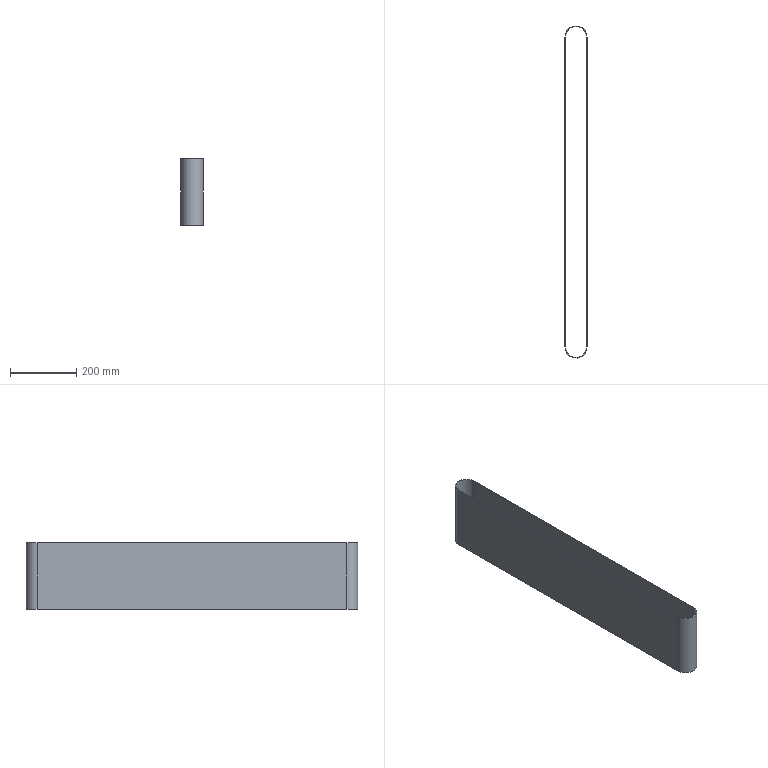Part | STEP file | MM-P41130-13_1 | 1 solid | 10 faces | box 67 x 999.5 x 200 mm | volume 621232 mm3 | plane 6 | cylinder 4 | commonest cylinder face diameters 64 x2 67 x2
STEP:
#1=CARTESIAN_POINT('',(0.,0.,0.));
#2=DIRECTION('',(0.,0.,1.));
#3=DIRECTION('',(1.,0.,0.));
#4=AXIS2_PLACEMENT_3D('',#1,#2,#3);
#5=CARTESIAN_POINT('',(-17.,-947.5,100.));
#6=VERTEX_POINT('',#5);
#7=CARTESIAN_POINT('',(-17.,-947.5,-100.));
#8=VERTEX_POINT('',#7);
#9=CARTESIAN_POINT('',(-17.,-947.5,100.));
#10=DIRECTION('',(0.,0.,-1.));
#11=VECTOR('',#10,1.);
#12=LINE('',#9,#11);
#13=CARTESIAN_POINT('',(-17.,-15.,100.));
#14=DIRECTION('',(1.,-0.000000039,0.));
#15=DIRECTION('',(0.000000039,1.,0.));
#16=AXIS2_PLACEMENT_3D('',#13,#14,#15);
#17=PLANE('',#16);
#18=CARTESIAN_POINT('',(-932.5,0.));
#19=DIRECTION('',(0.,-1.));
#20=VECTOR('',#19,1.);
#21=LINE('',#18,#20);
#22=(GEOMETRIC_REPRESENTATION_CONTEXT(2)PARAMETRIC_REPRESENTATION_CONTEXT()REPRESENTATION_CONTEXT('',''));
#23=DEFINITIONAL_REPRESENTATION('',(#21),#22);
#24=PCURVE('',#17,#23);
#25=CARTESIAN_POINT('',(16.5,-947.5,100.));
#26=DIRECTION('',(0.,0.,1.));
#27=DIRECTION('',(1.,0.,0.));
#28=AXIS2_PLACEMENT_3D('',#25,#26,#27);
#29=CYLINDRICAL_SURFACE('',#28,33.5);
#30=CARTESIAN_POINT('',(3.142,0.));
#31=DIRECTION('',(0.,-1.));
#32=VECTOR('',#31,1.);
#33=LINE('',#30,#32);
#34=(GEOMETRIC_REPRESENTATION_CONTEXT(2)PARAMETRIC_REPRESENTATION_CONTEXT()REPRESENTATION_CONTEXT('',''));
#35=DEFINITIONAL_REPRESENTATION('',(#33),#34);
#36=PCURVE('',#29,#35);
#37=SURFACE_CURVE('',#12,(#24,#36),.PCURVE_S1.);
#38=EDGE_CURVE('',#6,#8,#37,.T.);
#39=ORIENTED_EDGE('',*,*,#38,.F.);
#40=CARTESIAN_POINT('',(-17.,-15.,100.));
#41=VERTEX_POINT('',#40);
#42=CARTESIAN_POINT('',(-17.,-15.,100.));
#43=DIRECTION('',(-0.000000039,-1.,0.));
#44=VECTOR('',#43,1.);
#45=LINE('',#42,#44);
#46=CARTESIAN_POINT('',(0.,0.));
#47=DIRECTION('',(-1.,0.));
#48=VECTOR('',#47,1.);
#49=LINE('',#46,#48);
#50=(GEOMETRIC_REPRESENTATION_CONTEXT(2)PARAMETRIC_REPRESENTATION_CONTEXT()REPRESENTATION_CONTEXT('',''));
#51=DEFINITIONAL_REPRESENTATION('',(#49),#50);
#52=PCURVE('',#17,#51);
#53=CARTESIAN_POINT('',(16.5,-15.,100.));
#54=DIRECTION('',(0.,0.,-1.));
#55=DIRECTION('',(-1.,0.,0.));
#56=AXIS2_PLACEMENT_3D('',#53,#54,#55);
#57=PLANE('',#56);
#58=CARTESIAN_POINT('',(33.5,0.00000132));
#59=DIRECTION('',(0.000000039,-1.));
#60=VECTOR('',#59,1.);
#61=LINE('',#58,#60);
#62=(GEOMETRIC_REPRESENTATION_CONTEXT(2)PARAMETRIC_REPRESENTATION_CONTEXT()REPRESENTATION_CONTEXT('',''));
#63=DEFINITIONAL_REPRESENTATION('',(#61),#62);
#64=PCURVE('',#57,#63);
#65=SURFACE_CURVE('',#45,(#52,#64),.PCURVE_S1.);
#66=EDGE_CURVE('',#41,#6,#65,.T.);
#67=ORIENTED_EDGE('',*,*,#66,.F.);
#68=CARTESIAN_POINT('',(-17.,-15.,-100.));
#69=VERTEX_POINT('',#68);
#70=CARTESIAN_POINT('',(-17.,-15.,100.));
#71=DIRECTION('',(0.,0.,1.));
#72=VECTOR('',#71,1.);
#73=LINE('',#70,#72);
#74=CARTESIAN_POINT('',(0.,0.));
#75=DIRECTION('',(0.,1.));
#76=VECTOR('',#75,1.);
#77=LINE('',#74,#76);
#78=(GEOMETRIC_REPRESENTATION_CONTEXT(2)PARAMETRIC_REPRESENTATION_CONTEXT()REPRESENTATION_CONTEXT('',''));
#79=DEFINITIONAL_REPRESENTATION('',(#77),#78);
#80=PCURVE('',#17,#79);
#81=CARTESIAN_POINT('',(16.5,-15.,100.));
#82=DIRECTION('',(0.,0.,1.));
#83=DIRECTION('',(1.,0.,0.));
#84=AXIS2_PLACEMENT_3D('',#81,#82,#83);
#85=CYLINDRICAL_SURFACE('',#84,33.5);
#86=CARTESIAN_POINT('',(3.142,0.));
#87=DIRECTION('',(0.,1.));
#88=VECTOR('',#87,1.);
#89=LINE('',#86,#88);
#90=(GEOMETRIC_REPRESENTATION_CONTEXT(2)PARAMETRIC_REPRESENTATION_CONTEXT()REPRESENTATION_CONTEXT('',''));
#91=DEFINITIONAL_REPRESENTATION('',(#89),#90);
#92=PCURVE('',#85,#91);
#93=SURFACE_CURVE('',#73,(#80,#92),.PCURVE_S1.);
#94=EDGE_CURVE('',#69,#41,#93,.T.);
#95=ORIENTED_EDGE('',*,*,#94,.F.);
#96=CARTESIAN_POINT('',(-17.,-15.,-100.));
#97=DIRECTION('',(0.000000039,1.,0.));
#98=VECTOR('',#97,1.);
#99=LINE('',#96,#98);
#100=CARTESIAN_POINT('',(0.,-200.));
#101=DIRECTION('',(1.,0.));
#102=VECTOR('',#101,1.);
#103=LINE('',#100,#102);
#104=(GEOMETRIC_REPRESENTATION_CONTEXT(2)PARAMETRIC_REPRESENTATION_CONTEXT()REPRESENTATION_CONTEXT('',''));
#105=DEFINITIONAL_REPRESENTATION('',(#103),#104);
#106=PCURVE('',#17,#105);
#107=CARTESIAN_POINT('',(16.5,-15.,-100.));
#108=DIRECTION('',(0.,0.,-1.));
#109=DIRECTION('',(-1.,0.,0.));
#110=AXIS2_PLACEMENT_3D('',#107,#108,#109);
#111=PLANE('',#110);
#112=CARTESIAN_POINT('',(33.5,0.00000132));
#113=DIRECTION('',(-0.000000039,1.));
#114=VECTOR('',#113,1.);
#115=LINE('',#112,#114);
#116=(GEOMETRIC_REPRESENTATION_CONTEXT(2)PARAMETRIC_REPRESENTATION_CONTEXT()REPRESENTATION_CONTEXT('',''));
#117=DEFINITIONAL_REPRESENTATION('',(#115),#116);
#118=PCURVE('',#111,#117);
#119=SURFACE_CURVE('',#99,(#106,#118),.PCURVE_S1.);
#120=EDGE_CURVE('',#8,#69,#119,.T.);
#121=ORIENTED_EDGE('',*,*,#120,.F.);
#122=EDGE_LOOP('',(#39,#67,#95,#121));
#123=FACE_BOUND('',#122,.T.);
#124=ADVANCED_FACE('',(#123),#17,.F.);
#125=CARTESIAN_POINT('',(-15.5,-15.,-100.));
#126=VERTEX_POINT('',#125);
#127=CARTESIAN_POINT('',(-15.5,-947.5,-100.));
#128=VERTEX_POINT('',#127);
#129=CARTESIAN_POINT('',(-15.5,-15.,-100.));
#130=DIRECTION('',(-0.000000039,-1.,0.));
#131=VECTOR('',#130,1.);
#132=LINE('',#129,#131);
#133=CARTESIAN_POINT('',(32.,0.000001261));
#134=DIRECTION('',(0.000000039,-1.));
#135=VECTOR('',#134,1.);
#136=LINE('',#133,#135);
#137=(GEOMETRIC_REPRESENTATION_CONTEXT(2)PARAMETRIC_REPRESENTATION_CONTEXT()REPRESENTATION_CONTEXT('',''));
#138=DEFINITIONAL_REPRESENTATION('',(#136),#137);
#139=PCURVE('',#111,#138);
#140=CARTESIAN_POINT('',(-15.5,-947.5,100.));
#141=DIRECTION('',(1.,-0.000000039,0.));
#142=DIRECTION('',(0.000000039,1.,0.));
#143=AXIS2_PLACEMENT_3D('',#140,#141,#142);
#144=PLANE('',#143);
#145=CARTESIAN_POINT('',(932.5,-200.));
#146=DIRECTION('',(-1.,0.));
#147=VECTOR('',#146,1.);
#148=LINE('',#145,#147);
#149=(GEOMETRIC_REPRESENTATION_CONTEXT(2)PARAMETRIC_REPRESENTATION_CONTEXT()REPRESENTATION_CONTEXT('',''));
#150=DEFINITIONAL_REPRESENTATION('',(#148),#149);
#151=PCURVE('',#144,#150);
#152=SURFACE_CURVE('',#132,(#139,#151),.PCURVE_S1.);
#153=EDGE_CURVE('',#126,#128,#152,.T.);
#154=ORIENTED_EDGE('',*,*,#153,.T.);
#155=CARTESIAN_POINT('',(48.5,-947.5,-100.));
#156=VERTEX_POINT('',#155);
#157=CARTESIAN_POINT('',(16.5,-947.5,-100.));
#158=DIRECTION('',(0.,0.,1.));
#159=DIRECTION('',(1.,0.,0.));
#160=AXIS2_PLACEMENT_3D('',#157,#158,#159);
#161=CIRCLE('',#160,32.);
#162=CARTESIAN_POINT('',(-32.,-932.5));
#163=CARTESIAN_POINT('',(-32.,-877.074));
#164=CARTESIAN_POINT('',(16.,-904.787));
#165=CARTESIAN_POINT('',(64.,-932.5));
#166=CARTESIAN_POINT('',(16.,-960.213));
#167=CARTESIAN_POINT('',(-32.,-987.926));
#168=CARTESIAN_POINT('',(-32.,-932.5));
#169=(BOUNDED_CURVE()B_SPLINE_CURVE(2,(#162,#163,#164,#165,#166,#167,#168),.UNSPECIFIED.,.T.,.F.)B_SPLINE_CURVE_WITH_KNOTS((1,2,2,2,2,1),(-2.094,0.,2.094,4.189,6.283,8.378),.UNSPECIFIED.)CURVE()GEOMETRIC_REPRESENTATION_ITEM()RATIONAL_B_SPLINE_CURVE((1.,0.5,1.,0.5,1.,0.5,1.))REPRESENTATION_ITEM(''));
#170=(GEOMETRIC_REPRESENTATION_CONTEXT(2)PARAMETRIC_REPRESENTATION_CONTEXT()REPRESENTATION_CONTEXT('',''));
#171=DEFINITIONAL_REPRESENTATION('',(#169),#170);
#172=PCURVE('',#111,#171);
#173=CARTESIAN_POINT('',(16.5,-947.5,100.));
#174=DIRECTION('',(0.,0.,1.));
#175=DIRECTION('',(1.,0.,0.));
#176=AXIS2_PLACEMENT_3D('',#173,#174,#175);
#177=CYLINDRICAL_SURFACE('',#176,32.);
#178=CARTESIAN_POINT('',(0.,-200.));
#179=DIRECTION('',(1.,0.));
#180=VECTOR('',#179,1.);
#181=LINE('',#178,#180);
#182=(GEOMETRIC_REPRESENTATION_CONTEXT(2)PARAMETRIC_REPRESENTATION_CONTEXT()REPRESENTATION_CONTEXT('',''));
#183=DEFINITIONAL_REPRESENTATION('',(#181),#182);
#184=PCURVE('',#177,#183);
#185=SURFACE_CURVE('',#161,(#172,#184),.PCURVE_S1.);
#186=EDGE_CURVE('',#128,#156,#185,.T.);
#187=ORIENTED_EDGE('',*,*,#186,.T.);
#188=CARTESIAN_POINT('',(48.5,-15.,-100.));
#189=VERTEX_POINT('',#188);
#190=CARTESIAN_POINT('',(48.5,-947.5,-100.));
#191=DIRECTION('',(0.000000039,1.,0.));
#192=VECTOR('',#191,1.);
#193=LINE('',#190,#192);
#194=CARTESIAN_POINT('',(-32.,-932.5));
#195=DIRECTION('',(-0.000000039,1.));
#196=VECTOR('',#195,1.);
#197=LINE('',#194,#196);
#198=(GEOMETRIC_REPRESENTATION_CONTEXT(2)PARAMETRIC_REPRESENTATION_CONTEXT()REPRESENTATION_CONTEXT('',''));
#199=DEFINITIONAL_REPRESENTATION('',(#197),#198);
#200=PCURVE('',#111,#199);
#201=CARTESIAN_POINT('',(48.5,-15.,100.));
#202=DIRECTION('',(-1.,0.000000039,0.));
#203=DIRECTION('',(-0.000000039,-1.,0.));
#204=AXIS2_PLACEMENT_3D('',#201,#202,#203);
#205=PLANE('',#204);
#206=CARTESIAN_POINT('',(932.5,-200.));
#207=DIRECTION('',(-1.,0.));
#208=VECTOR('',#207,1.);
#209=LINE('',#206,#208);
#210=(GEOMETRIC_REPRESENTATION_CONTEXT(2)PARAMETRIC_REPRESENTATION_CONTEXT()REPRESENTATION_CONTEXT('',''));
#211=DEFINITIONAL_REPRESENTATION('',(#209),#210);
#212=PCURVE('',#205,#211);
#213=SURFACE_CURVE('',#193,(#200,#212),.PCURVE_S1.);
#214=EDGE_CURVE('',#156,#189,#213,.T.);
#215=ORIENTED_EDGE('',*,*,#214,.T.);
#216=CARTESIAN_POINT('',(16.5,-15.,-100.));
#217=DIRECTION('',(0.,0.,1.));
#218=DIRECTION('',(1.,0.,0.));
#219=AXIS2_PLACEMENT_3D('',#216,#217,#218);
#220=CIRCLE('',#219,32.);
#221=CARTESIAN_POINT('',(-32.,0.));
#222=CARTESIAN_POINT('',(-32.,55.426));
#223=CARTESIAN_POINT('',(16.,27.713));
#224=CARTESIAN_POINT('',(64.,0.));
#225=CARTESIAN_POINT('',(16.,-27.713));
#226=CARTESIAN_POINT('',(-32.,-55.426));
#227=CARTESIAN_POINT('',(-32.,0.));
#228=(BOUNDED_CURVE()B_SPLINE_CURVE(2,(#221,#222,#223,#224,#225,#226,#227),.UNSPECIFIED.,.T.,.F.)B_SPLINE_CURVE_WITH_KNOTS((1,2,2,2,2,1),(-2.094,0.,2.094,4.189,6.283,8.378),.UNSPECIFIED.)CURVE()GEOMETRIC_REPRESENTATION_ITEM()RATIONAL_B_SPLINE_CURVE((1.,0.5,1.,0.5,1.,0.5,1.))REPRESENTATION_ITEM(''));
#229=(GEOMETRIC_REPRESENTATION_CONTEXT(2)PARAMETRIC_REPRESENTATION_CONTEXT()REPRESENTATION_CONTEXT('',''));
#230=DEFINITIONAL_REPRESENTATION('',(#228),#229);
#231=PCURVE('',#111,#230);
#232=CARTESIAN_POINT('',(16.5,-15.,100.));
#233=DIRECTION('',(0.,0.,1.));
#234=DIRECTION('',(1.,0.,0.));
#235=AXIS2_PLACEMENT_3D('',#232,#233,#234);
#236=CYLINDRICAL_SURFACE('',#235,32.);
#237=CARTESIAN_POINT('',(-6.283,-200.));
#238=DIRECTION('',(1.,0.));
#239=VECTOR('',#238,1.);
#240=LINE('',#237,#239);
#241=(GEOMETRIC_REPRESENTATION_CONTEXT(2)PARAMETRIC_REPRESENTATION_CONTEXT()REPRESENTATION_CONTEXT('',''));
#242=DEFINITIONAL_REPRESENTATION('',(#240),#241);
#243=PCURVE('',#236,#242);
#244=SURFACE_CURVE('',#220,(#231,#243),.PCURVE_S1.);
#245=EDGE_CURVE('',#189,#126,#244,.T.);
#246=ORIENTED_EDGE('',*,*,#245,.T.);
#247=EDGE_LOOP('',(#154,#187,#215,#246));
#248=FACE_BOUND('',#247,.T.);
#249=CARTESIAN_POINT('',(50.,-947.5,-100.));
#250=VERTEX_POINT('',#249);
#251=CARTESIAN_POINT('',(16.5,-947.5,-100.));
#252=DIRECTION('',(0.,0.,-1.));
#253=DIRECTION('',(1.,0.,0.));
#254=AXIS2_PLACEMENT_3D('',#251,#252,#253);
#255=CIRCLE('',#254,33.5);
#256=CARTESIAN_POINT('',(0.00003674,-932.5));
#257=DIRECTION('',(-1.,0.));
#258=AXIS2_PLACEMENT_2D('',#256,#257);
#259=CIRCLE('',#258,33.5);
#260=(GEOMETRIC_REPRESENTATION_CONTEXT(2)PARAMETRIC_REPRESENTATION_CONTEXT()REPRESENTATION_CONTEXT('',''));
#261=DEFINITIONAL_REPRESENTATION('',(#259),#260);
#262=PCURVE('',#111,#261);
#263=CARTESIAN_POINT('',(6.283,-200.));
#264=DIRECTION('',(-1.,0.));
#265=VECTOR('',#264,1.);
#266=LINE('',#263,#265);
#267=(GEOMETRIC_REPRESENTATION_CONTEXT(2)PARAMETRIC_REPRESENTATION_CONTEXT()REPRESENTATION_CONTEXT('',''));
#268=DEFINITIONAL_REPRESENTATION('',(#266),#267);
#269=PCURVE('',#29,#268);
#270=SURFACE_CURVE('',#255,(#262,#269),.PCURVE_S1.);
#271=EDGE_CURVE('',#250,#8,#270,.T.);
#272=ORIENTED_EDGE('',*,*,#271,.T.);
#273=ORIENTED_EDGE('',*,*,#120,.T.);
#274=CARTESIAN_POINT('',(50.,-15.,-100.));
#275=VERTEX_POINT('',#274);
#276=CARTESIAN_POINT('',(16.5,-15.,-100.));
#277=DIRECTION('',(0.,0.,-1.));
#278=DIRECTION('',(1.,0.,0.));
#279=AXIS2_PLACEMENT_3D('',#276,#277,#278);
#280=CIRCLE('',#279,33.5);
#281=CARTESIAN_POINT('',(0.,0.));
#282=DIRECTION('',(-1.,0.));
#283=AXIS2_PLACEMENT_2D('',#281,#282);
#284=CIRCLE('',#283,33.5);
#285=(GEOMETRIC_REPRESENTATION_CONTEXT(2)PARAMETRIC_REPRESENTATION_CONTEXT()REPRESENTATION_CONTEXT('',''));
#286=DEFINITIONAL_REPRESENTATION('',(#284),#285);
#287=PCURVE('',#111,#286);
#288=CARTESIAN_POINT('',(6.283,-200.));
#289=DIRECTION('',(-1.,0.));
#290=VECTOR('',#289,1.);
#291=LINE('',#288,#290);
#292=(GEOMETRIC_REPRESENTATION_CONTEXT(2)PARAMETRIC_REPRESENTATION_CONTEXT()REPRESENTATION_CONTEXT('',''));
#293=DEFINITIONAL_REPRESENTATION('',(#291),#292);
#294=PCURVE('',#85,#293);
#295=SURFACE_CURVE('',#280,(#287,#294),.PCURVE_S1.);
#296=EDGE_CURVE('',#69,#275,#295,.T.);
#297=ORIENTED_EDGE('',*,*,#296,.T.);
#298=CARTESIAN_POINT('',(50.,-15.,-100.));
#299=DIRECTION('',(-0.000000039,-1.,0.));
#300=VECTOR('',#299,1.);
#301=LINE('',#298,#300);
#302=CARTESIAN_POINT('',(-33.5,-0.00000132));
#303=DIRECTION('',(0.000000039,-1.));
#304=VECTOR('',#303,1.);
#305=LINE('',#302,#304);
#306=(GEOMETRIC_REPRESENTATION_CONTEXT(2)PARAMETRIC_REPRESENTATION_CONTEXT()REPRESENTATION_CONTEXT('',''));
#307=DEFINITIONAL_REPRESENTATION('',(#305),#306);
#308=PCURVE('',#111,#307);
#309=CARTESIAN_POINT('',(50.,-15.,100.));
#310=DIRECTION('',(-1.,0.000000039,0.));
#311=DIRECTION('',(-0.000000039,-1.,0.));
#312=AXIS2_PLACEMENT_3D('',#309,#310,#311);
#313=PLANE('',#312);
#314=CARTESIAN_POINT('',(0.,-200.));
#315=DIRECTION('',(1.,0.));
#316=VECTOR('',#315,1.);
#317=LINE('',#314,#316);
#318=(GEOMETRIC_REPRESENTATION_CONTEXT(2)PARAMETRIC_REPRESENTATION_CONTEXT()REPRESENTATION_CONTEXT('',''));
#319=DEFINITIONAL_REPRESENTATION('',(#317),#318);
#320=PCURVE('',#313,#319);
#321=SURFACE_CURVE('',#301,(#308,#320),.PCURVE_S1.);
#322=EDGE_CURVE('',#275,#250,#321,.T.);
#323=ORIENTED_EDGE('',*,*,#322,.T.);
#324=EDGE_LOOP('',(#272,#273,#297,#323));
#325=FACE_BOUND('',#324,.T.);
#326=ADVANCED_FACE('',(#248,#325),#111,.T.);
#327=CARTESIAN_POINT('',(50.,-947.5,100.));
#328=VERTEX_POINT('',#327);
#329=CARTESIAN_POINT('',(16.5,-947.5,100.));
#330=DIRECTION('',(0.,0.,-1.));
#331=DIRECTION('',(1.,0.,0.));
#332=AXIS2_PLACEMENT_3D('',#329,#330,#331);
#333=CIRCLE('',#332,33.5);
#334=CARTESIAN_POINT('',(6.283,0.));
#335=DIRECTION('',(-1.,0.));
#336=VECTOR('',#335,1.);
#337=LINE('',#334,#336);
#338=(GEOMETRIC_REPRESENTATION_CONTEXT(2)PARAMETRIC_REPRESENTATION_CONTEXT()REPRESENTATION_CONTEXT('',''));
#339=DEFINITIONAL_REPRESENTATION('',(#337),#338);
#340=PCURVE('',#29,#339);
#341=CARTESIAN_POINT('',(0.00003674,-932.5));
#342=DIRECTION('',(-1.,0.));
#343=AXIS2_PLACEMENT_2D('',#341,#342);
#344=CIRCLE('',#343,33.5);
#345=(GEOMETRIC_REPRESENTATION_CONTEXT(2)PARAMETRIC_REPRESENTATION_CONTEXT()REPRESENTATION_CONTEXT('',''));
#346=DEFINITIONAL_REPRESENTATION('',(#344),#345);
#347=PCURVE('',#57,#346);
#348=SURFACE_CURVE('',#333,(#340,#347),.PCURVE_S1.);
#349=EDGE_CURVE('',#328,#6,#348,.T.);
#350=ORIENTED_EDGE('',*,*,#349,.T.);
#351=ORIENTED_EDGE('',*,*,#38,.T.);
#352=ORIENTED_EDGE('',*,*,#271,.F.);
#353=CARTESIAN_POINT('',(50.,-947.5,100.));
#354=DIRECTION('',(0.,0.,1.));
#355=VECTOR('',#354,1.);
#356=LINE('',#353,#355);
#357=CARTESIAN_POINT('',(6.283,0.));
#358=DIRECTION('',(0.,1.));
#359=VECTOR('',#358,1.);
#360=LINE('',#357,#359);
#361=(GEOMETRIC_REPRESENTATION_CONTEXT(2)PARAMETRIC_REPRESENTATION_CONTEXT()REPRESENTATION_CONTEXT('',''));
#362=DEFINITIONAL_REPRESENTATION('',(#360),#361);
#363=PCURVE('',#29,#362);
#364=CARTESIAN_POINT('',(932.5,0.));
#365=DIRECTION('',(0.,1.));
#366=VECTOR('',#365,1.);
#367=LINE('',#364,#366);
#368=(GEOMETRIC_REPRESENTATION_CONTEXT(2)PARAMETRIC_REPRESENTATION_CONTEXT()REPRESENTATION_CONTEXT('',''));
#369=DEFINITIONAL_REPRESENTATION('',(#367),#368);
#370=PCURVE('',#313,#369);
#371=SURFACE_CURVE('',#356,(#363,#370),.PCURVE_S1.);
#372=EDGE_CURVE('',#250,#328,#371,.T.);
#373=ORIENTED_EDGE('',*,*,#372,.T.);
#374=EDGE_LOOP('',(#350,#351,#352,#373));
#375=FACE_BOUND('',#374,.T.);
#376=ADVANCED_FACE('',(#375),#29,.T.);
#377=CARTESIAN_POINT('',(48.5,-947.5,100.));
#378=VERTEX_POINT('',#377);
#379=CARTESIAN_POINT('',(48.5,-15.,100.));
#380=VERTEX_POINT('',#379);
#381=CARTESIAN_POINT('',(48.5,-947.5,100.));
#382=DIRECTION('',(0.000000039,1.,0.));
#383=VECTOR('',#382,1.);
#384=LINE('',#381,#383);
#385=CARTESIAN_POINT('',(-32.,-932.5));
#386=DIRECTION('',(-0.000000039,1.));
#387=VECTOR('',#386,1.);
#388=LINE('',#385,#387);
#389=(GEOMETRIC_REPRESENTATION_CONTEXT(2)PARAMETRIC_REPRESENTATION_CONTEXT()REPRESENTATION_CONTEXT('',''));
#390=DEFINITIONAL_REPRESENTATION('',(#388),#389);
#391=PCURVE('',#57,#390);
#392=CARTESIAN_POINT('',(932.5,0.));
#393=DIRECTION('',(-1.,0.));
#394=VECTOR('',#393,1.);
#395=LINE('',#392,#394);
#396=(GEOMETRIC_REPRESENTATION_CONTEXT(2)PARAMETRIC_REPRESENTATION_CONTEXT()REPRESENTATION_CONTEXT('',''));
#397=DEFINITIONAL_REPRESENTATION('',(#395),#396);
#398=PCURVE('',#205,#397);
#399=SURFACE_CURVE('',#384,(#391,#398),.PCURVE_S1.);
#400=EDGE_CURVE('',#378,#380,#399,.T.);
#401=ORIENTED_EDGE('',*,*,#400,.F.);
#402=CARTESIAN_POINT('',(-15.5,-947.5,100.));
#403=VERTEX_POINT('',#402);
#404=CARTESIAN_POINT('',(16.5,-947.5,100.));
#405=DIRECTION('',(0.,0.,1.));
#406=DIRECTION('',(1.,0.,0.));
#407=AXIS2_PLACEMENT_3D('',#404,#405,#406);
#408=CIRCLE('',#407,32.);
#409=CARTESIAN_POINT('',(-32.,-932.5));
#410=CARTESIAN_POINT('',(-32.,-877.074));
#411=CARTESIAN_POINT('',(16.,-904.787));
#412=CARTESIAN_POINT('',(64.,-932.5));
#413=CARTESIAN_POINT('',(16.,-960.213));
#414=CARTESIAN_POINT('',(-32.,-987.926));
#415=CARTESIAN_POINT('',(-32.,-932.5));
#416=(BOUNDED_CURVE()B_SPLINE_CURVE(2,(#409,#410,#411,#412,#413,#414,#415),.UNSPECIFIED.,.T.,.F.)B_SPLINE_CURVE_WITH_KNOTS((1,2,2,2,2,1),(-2.094,0.,2.094,4.189,6.283,8.378),.UNSPECIFIED.)CURVE()GEOMETRIC_REPRESENTATION_ITEM()RATIONAL_B_SPLINE_CURVE((1.,0.5,1.,0.5,1.,0.5,1.))REPRESENTATION_ITEM(''));
#417=(GEOMETRIC_REPRESENTATION_CONTEXT(2)PARAMETRIC_REPRESENTATION_CONTEXT()REPRESENTATION_CONTEXT('',''));
#418=DEFINITIONAL_REPRESENTATION('',(#416),#417);
#419=PCURVE('',#57,#418);
#420=CARTESIAN_POINT('',(0.,0.));
#421=DIRECTION('',(1.,0.));
#422=VECTOR('',#421,1.);
#423=LINE('',#420,#422);
#424=(GEOMETRIC_REPRESENTATION_CONTEXT(2)PARAMETRIC_REPRESENTATION_CONTEXT()REPRESENTATION_CONTEXT('',''));
#425=DEFINITIONAL_REPRESENTATION('',(#423),#424);
#426=PCURVE('',#177,#425);
#427=SURFACE_CURVE('',#408,(#419,#426),.PCURVE_S1.);
#428=EDGE_CURVE('',#403,#378,#427,.T.);
#429=ORIENTED_EDGE('',*,*,#428,.F.);
#430=CARTESIAN_POINT('',(-15.5,-15.,100.));
#431=VERTEX_POINT('',#430);
#432=CARTESIAN_POINT('',(-15.5,-15.,100.));
#433=DIRECTION('',(-0.000000039,-1.,0.));
#434=VECTOR('',#433,1.);
#435=LINE('',#432,#434);
#436=CARTESIAN_POINT('',(32.,0.000001261));
#437=DIRECTION('',(0.000000039,-1.));
#438=VECTOR('',#437,1.);
#439=LINE('',#436,#438);
#440=(GEOMETRIC_REPRESENTATION_CONTEXT(2)PARAMETRIC_REPRESENTATION_CONTEXT()REPRESENTATION_CONTEXT('',''));
#441=DEFINITIONAL_REPRESENTATION('',(#439),#440);
#442=PCURVE('',#57,#441);
#443=CARTESIAN_POINT('',(932.5,0.));
#444=DIRECTION('',(-1.,0.));
#445=VECTOR('',#444,1.);
#446=LINE('',#443,#445);
#447=(GEOMETRIC_REPRESENTATION_CONTEXT(2)PARAMETRIC_REPRESENTATION_CONTEXT()REPRESENTATION_CONTEXT('',''));
#448=DEFINITIONAL_REPRESENTATION('',(#446),#447);
#449=PCURVE('',#144,#448);
#450=SURFACE_CURVE('',#435,(#442,#449),.PCURVE_S1.);
#451=EDGE_CURVE('',#431,#403,#450,.T.);
#452=ORIENTED_EDGE('',*,*,#451,.F.);
#453=CARTESIAN_POINT('',(16.5,-15.,100.));
#454=DIRECTION('',(0.,0.,1.));
#455=DIRECTION('',(1.,0.,0.));
#456=AXIS2_PLACEMENT_3D('',#453,#454,#455);
#457=CIRCLE('',#456,32.);
#458=CARTESIAN_POINT('',(-32.,0.));
#459=CARTESIAN_POINT('',(-32.,55.426));
#460=CARTESIAN_POINT('',(16.,27.713));
#461=CARTESIAN_POINT('',(64.,0.));
#462=CARTESIAN_POINT('',(16.,-27.713));
#463=CARTESIAN_POINT('',(-32.,-55.426));
#464=CARTESIAN_POINT('',(-32.,0.));
#465=(BOUNDED_CURVE()B_SPLINE_CURVE(2,(#458,#459,#460,#461,#462,#463,#464),.UNSPECIFIED.,.T.,.F.)B_SPLINE_CURVE_WITH_KNOTS((1,2,2,2,2,1),(-2.094,0.,2.094,4.189,6.283,8.378),.UNSPECIFIED.)CURVE()GEOMETRIC_REPRESENTATION_ITEM()RATIONAL_B_SPLINE_CURVE((1.,0.5,1.,0.5,1.,0.5,1.))REPRESENTATION_ITEM(''));
#466=(GEOMETRIC_REPRESENTATION_CONTEXT(2)PARAMETRIC_REPRESENTATION_CONTEXT()REPRESENTATION_CONTEXT('',''));
#467=DEFINITIONAL_REPRESENTATION('',(#465),#466);
#468=PCURVE('',#57,#467);
#469=CARTESIAN_POINT('',(-6.283,0.));
#470=DIRECTION('',(1.,0.));
#471=VECTOR('',#470,1.);
#472=LINE('',#469,#471);
#473=(GEOMETRIC_REPRESENTATION_CONTEXT(2)PARAMETRIC_REPRESENTATION_CONTEXT()REPRESENTATION_CONTEXT('',''));
#474=DEFINITIONAL_REPRESENTATION('',(#472),#473);
#475=PCURVE('',#236,#474);
#476=SURFACE_CURVE('',#457,(#468,#475),.PCURVE_S1.);
#477=EDGE_CURVE('',#380,#431,#476,.T.);
#478=ORIENTED_EDGE('',*,*,#477,.F.);
#479=EDGE_LOOP('',(#401,#429,#452,#478));
#480=FACE_BOUND('',#479,.T.);
#481=ORIENTED_EDGE('',*,*,#66,.T.);
#482=ORIENTED_EDGE('',*,*,#349,.F.);
#483=CARTESIAN_POINT('',(50.,-15.,100.));
#484=VERTEX_POINT('',#483);
#485=CARTESIAN_POINT('',(50.,-15.,100.));
#486=DIRECTION('',(-0.000000039,-1.,0.));
#487=VECTOR('',#486,1.);
#488=LINE('',#485,#487);
#489=CARTESIAN_POINT('',(-33.5,-0.00000132));
#490=DIRECTION('',(0.000000039,-1.));
#491=VECTOR('',#490,1.);
#492=LINE('',#489,#491);
#493=(GEOMETRIC_REPRESENTATION_CONTEXT(2)PARAMETRIC_REPRESENTATION_CONTEXT()REPRESENTATION_CONTEXT('',''));
#494=DEFINITIONAL_REPRESENTATION('',(#492),#493);
#495=PCURVE('',#57,#494);
#496=CARTESIAN_POINT('',(0.,0.));
#497=DIRECTION('',(1.,0.));
#498=VECTOR('',#497,1.);
#499=LINE('',#496,#498);
#500=(GEOMETRIC_REPRESENTATION_CONTEXT(2)PARAMETRIC_REPRESENTATION_CONTEXT()REPRESENTATION_CONTEXT('',''));
#501=DEFINITIONAL_REPRESENTATION('',(#499),#500);
#502=PCURVE('',#313,#501);
#503=SURFACE_CURVE('',#488,(#495,#502),.PCURVE_S1.);
#504=EDGE_CURVE('',#484,#328,#503,.T.);
#505=ORIENTED_EDGE('',*,*,#504,.F.);
#506=CARTESIAN_POINT('',(16.5,-15.,100.));
#507=DIRECTION('',(0.,0.,-1.));
#508=DIRECTION('',(1.,0.,0.));
#509=AXIS2_PLACEMENT_3D('',#506,#507,#508);
#510=CIRCLE('',#509,33.5);
#511=CARTESIAN_POINT('',(0.,0.));
#512=DIRECTION('',(-1.,0.));
#513=AXIS2_PLACEMENT_2D('',#511,#512);
#514=CIRCLE('',#513,33.5);
#515=(GEOMETRIC_REPRESENTATION_CONTEXT(2)PARAMETRIC_REPRESENTATION_CONTEXT()REPRESENTATION_CONTEXT('',''));
#516=DEFINITIONAL_REPRESENTATION('',(#514),#515);
#517=PCURVE('',#57,#516);
#518=CARTESIAN_POINT('',(6.283,0.));
#519=DIRECTION('',(-1.,0.));
#520=VECTOR('',#519,1.);
#521=LINE('',#518,#520);
#522=(GEOMETRIC_REPRESENTATION_CONTEXT(2)PARAMETRIC_REPRESENTATION_CONTEXT()REPRESENTATION_CONTEXT('',''));
#523=DEFINITIONAL_REPRESENTATION('',(#521),#522);
#524=PCURVE('',#85,#523);
#525=SURFACE_CURVE('',#510,(#517,#524),.PCURVE_S1.);
#526=EDGE_CURVE('',#41,#484,#525,.T.);
#527=ORIENTED_EDGE('',*,*,#526,.F.);
#528=EDGE_LOOP('',(#481,#482,#505,#527));
#529=FACE_BOUND('',#528,.T.);
#530=ADVANCED_FACE('',(#480,#529),#57,.F.);
#531=ORIENTED_EDGE('',*,*,#526,.T.);
#532=CARTESIAN_POINT('',(50.,-15.,100.));
#533=DIRECTION('',(0.,0.,-1.));
#534=VECTOR('',#533,1.);
#535=LINE('',#532,#534);
#536=CARTESIAN_POINT('',(0.,0.));
#537=DIRECTION('',(0.,-1.));
#538=VECTOR('',#537,1.);
#539=LINE('',#536,#538);
#540=(GEOMETRIC_REPRESENTATION_CONTEXT(2)PARAMETRIC_REPRESENTATION_CONTEXT()REPRESENTATION_CONTEXT('',''));
#541=DEFINITIONAL_REPRESENTATION('',(#539),#540);
#542=PCURVE('',#85,#541);
#543=CARTESIAN_POINT('',(-0.00000132,0.));
#544=DIRECTION('',(0.,-1.));
#545=VECTOR('',#544,1.);
#546=LINE('',#543,#545);
#547=(GEOMETRIC_REPRESENTATION_CONTEXT(2)PARAMETRIC_REPRESENTATION_CONTEXT()REPRESENTATION_CONTEXT('',''));
#548=DEFINITIONAL_REPRESENTATION('',(#546),#547);
#549=PCURVE('',#313,#548);
#550=SURFACE_CURVE('',#535,(#542,#549),.PCURVE_S1.);
#551=EDGE_CURVE('',#484,#275,#550,.T.);
#552=ORIENTED_EDGE('',*,*,#551,.T.);
#553=ORIENTED_EDGE('',*,*,#296,.F.);
#554=ORIENTED_EDGE('',*,*,#94,.T.);
#555=EDGE_LOOP('',(#531,#552,#553,#554));
#556=FACE_BOUND('',#555,.T.);
#557=ADVANCED_FACE('',(#556),#85,.T.);
#558=ORIENTED_EDGE('',*,*,#186,.T.);
#559=CARTESIAN_POINT('',(48.5,-947.5,100.));
#560=DIRECTION('',(0.,0.,1.));
#561=VECTOR('',#560,1.);
#562=LINE('',#559,#561);
#563=CARTESIAN_POINT('',(6.283,0.));
#564=DIRECTION('',(0.,1.));
#565=VECTOR('',#564,1.);
#566=LINE('',#563,#565);
#567=(GEOMETRIC_REPRESENTATION_CONTEXT(2)PARAMETRIC_REPRESENTATION_CONTEXT()REPRESENTATION_CONTEXT('',''));
#568=DEFINITIONAL_REPRESENTATION('',(#566),#567);
#569=PCURVE('',#177,#568);
#570=CARTESIAN_POINT('',(932.5,0.));
#571=DIRECTION('',(0.,1.));
#572=VECTOR('',#571,1.);
#573=LINE('',#570,#572);
#574=(GEOMETRIC_REPRESENTATION_CONTEXT(2)PARAMETRIC_REPRESENTATION_CONTEXT()REPRESENTATION_CONTEXT('',''));
#575=DEFINITIONAL_REPRESENTATION('',(#573),#574);
#576=PCURVE('',#205,#575);
#577=SURFACE_CURVE('',#562,(#569,#576),.PCURVE_S1.);
#578=EDGE_CURVE('',#156,#378,#577,.T.);
#579=ORIENTED_EDGE('',*,*,#578,.T.);
#580=ORIENTED_EDGE('',*,*,#428,.F.);
#581=CARTESIAN_POINT('',(-15.5,-947.5,100.));
#582=DIRECTION('',(0.,0.,-1.));
#583=VECTOR('',#582,1.);
#584=LINE('',#581,#583);
#585=CARTESIAN_POINT('',(3.142,0.));
#586=DIRECTION('',(0.,-1.));
#587=VECTOR('',#586,1.);
#588=LINE('',#585,#587);
#589=(GEOMETRIC_REPRESENTATION_CONTEXT(2)PARAMETRIC_REPRESENTATION_CONTEXT()REPRESENTATION_CONTEXT('',''));
#590=DEFINITIONAL_REPRESENTATION('',(#588),#589);
#591=PCURVE('',#177,#590);
#592=CARTESIAN_POINT('',(0.,0.));
#593=DIRECTION('',(0.,-1.));
#594=VECTOR('',#593,1.);
#595=LINE('',#592,#594);
#596=(GEOMETRIC_REPRESENTATION_CONTEXT(2)PARAMETRIC_REPRESENTATION_CONTEXT()REPRESENTATION_CONTEXT('',''));
#597=DEFINITIONAL_REPRESENTATION('',(#595),#596);
#598=PCURVE('',#144,#597);
#599=SURFACE_CURVE('',#584,(#591,#598),.PCURVE_S1.);
#600=EDGE_CURVE('',#403,#128,#599,.T.);
#601=ORIENTED_EDGE('',*,*,#600,.T.);
#602=EDGE_LOOP('',(#558,#579,#580,#601));
#603=FACE_BOUND('',#602,.F.);
#604=ADVANCED_FACE('',(#603),#177,.F.);
#605=ORIENTED_EDGE('',*,*,#451,.T.);
#606=ORIENTED_EDGE('',*,*,#600,.T.);
#607=ORIENTED_EDGE('',*,*,#153,.F.);
#608=CARTESIAN_POINT('',(-15.5,-15.,100.));
#609=DIRECTION('',(0.,0.,1.));
#610=VECTOR('',#609,1.);
#611=LINE('',#608,#610);
#612=CARTESIAN_POINT('',(932.5,0.));
#613=DIRECTION('',(0.,1.));
#614=VECTOR('',#613,1.);
#615=LINE('',#612,#614);
#616=(GEOMETRIC_REPRESENTATION_CONTEXT(2)PARAMETRIC_REPRESENTATION_CONTEXT()REPRESENTATION_CONTEXT('',''));
#617=DEFINITIONAL_REPRESENTATION('',(#615),#616);
#618=PCURVE('',#144,#617);
#619=CARTESIAN_POINT('',(3.142,0.));
#620=DIRECTION('',(0.,1.));
#621=VECTOR('',#620,1.);
#622=LINE('',#619,#621);
#623=(GEOMETRIC_REPRESENTATION_CONTEXT(2)PARAMETRIC_REPRESENTATION_CONTEXT()REPRESENTATION_CONTEXT('',''));
#624=DEFINITIONAL_REPRESENTATION('',(#622),#623);
#625=PCURVE('',#236,#624);
#626=SURFACE_CURVE('',#611,(#618,#625),.PCURVE_S1.);
#627=EDGE_CURVE('',#126,#431,#626,.T.);
#628=ORIENTED_EDGE('',*,*,#627,.T.);
#629=EDGE_LOOP('',(#605,#606,#607,#628));
#630=FACE_BOUND('',#629,.T.);
#631=ADVANCED_FACE('',(#630),#144,.T.);
#632=ORIENTED_EDGE('',*,*,#245,.T.);
#633=ORIENTED_EDGE('',*,*,#627,.T.);
#634=ORIENTED_EDGE('',*,*,#477,.F.);
#635=CARTESIAN_POINT('',(48.5,-15.,100.));
#636=DIRECTION('',(0.,0.,-1.));
#637=VECTOR('',#636,1.);
#638=LINE('',#635,#637);
#639=CARTESIAN_POINT('',(0.,0.));
#640=DIRECTION('',(0.,-1.));
#641=VECTOR('',#640,1.);
#642=LINE('',#639,#641);
#643=(GEOMETRIC_REPRESENTATION_CONTEXT(2)PARAMETRIC_REPRESENTATION_CONTEXT()REPRESENTATION_CONTEXT('',''));
#644=DEFINITIONAL_REPRESENTATION('',(#642),#643);
#645=PCURVE('',#236,#644);
#646=CARTESIAN_POINT('',(-0.000001261,0.));
#647=DIRECTION('',(0.,-1.));
#648=VECTOR('',#647,1.);
#649=LINE('',#646,#648);
#650=(GEOMETRIC_REPRESENTATION_CONTEXT(2)PARAMETRIC_REPRESENTATION_CONTEXT()REPRESENTATION_CONTEXT('',''));
#651=DEFINITIONAL_REPRESENTATION('',(#649),#650);
#652=PCURVE('',#205,#651);
#653=SURFACE_CURVE('',#638,(#645,#652),.PCURVE_S1.);
#654=EDGE_CURVE('',#380,#189,#653,.T.);
#655=ORIENTED_EDGE('',*,*,#654,.T.);
#656=EDGE_LOOP('',(#632,#633,#634,#655));
#657=FACE_BOUND('',#656,.F.);
#658=ADVANCED_FACE('',(#657),#236,.F.);
#659=ORIENTED_EDGE('',*,*,#400,.T.);
#660=ORIENTED_EDGE('',*,*,#654,.T.);
#661=ORIENTED_EDGE('',*,*,#214,.F.);
#662=ORIENTED_EDGE('',*,*,#578,.T.);
#663=EDGE_LOOP('',(#659,#660,#661,#662));
#664=FACE_BOUND('',#663,.T.);
#665=ADVANCED_FACE('',(#664),#205,.T.);
#666=ORIENTED_EDGE('',*,*,#551,.F.);
#667=ORIENTED_EDGE('',*,*,#504,.T.);
#668=ORIENTED_EDGE('',*,*,#372,.F.);
#669=ORIENTED_EDGE('',*,*,#322,.F.);
#670=EDGE_LOOP('',(#666,#667,#668,#669));
#671=FACE_BOUND('',#670,.T.);
#672=ADVANCED_FACE('',(#671),#313,.F.);
#673=CLOSED_SHELL('',(#124,#326,#376,#530,#557,#604,#631,#658,#665,#672));
#674=MANIFOLD_SOLID_BREP('',#673);
#675=(LENGTH_UNIT()NAMED_UNIT(*)SI_UNIT(.MILLI.,.METRE.));
#676=UNCERTAINTY_MEASURE_WITH_UNIT(LENGTH_MEASURE(0.0000002),#675,'','');
#677=(NAMED_UNIT(*)PLANE_ANGLE_UNIT()SI_UNIT($,.RADIAN.));
#678=(NAMED_UNIT(*)SI_UNIT($,.STERADIAN.)SOLID_ANGLE_UNIT());
#679=(GEOMETRIC_REPRESENTATION_CONTEXT(3)GLOBAL_UNCERTAINTY_ASSIGNED_CONTEXT((#676))GLOBAL_UNIT_ASSIGNED_CONTEXT((#675,#677,#678))REPRESENTATION_CONTEXT('',''));
#680=ADVANCED_BREP_SHAPE_REPRESENTATION('',(#4,#674),#679);